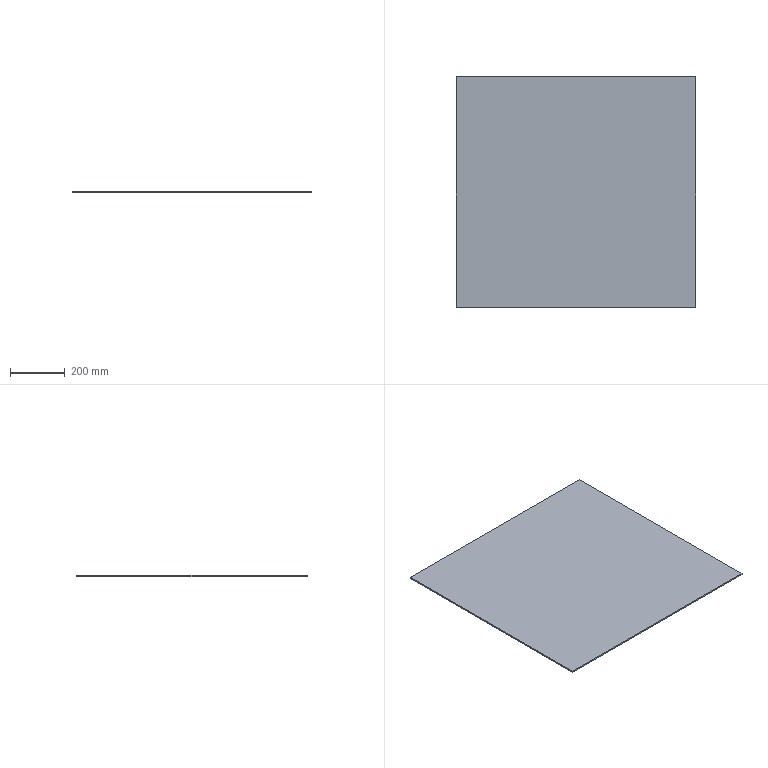Part | SolidWorks | features Extrusion 1, HoleWzd 1 | 1 solid | 6 faces | box 876 x 842 x 5 mm | volume 3687960 mm3 | plane 6
STEP:
#1=CARTESIAN_POINT('',(438.,-421.,0.));
#2=VERTEX_POINT('',#1);
#3=CARTESIAN_POINT('',(438.,421.,0.));
#4=VERTEX_POINT('',#3);
#5=CARTESIAN_POINT('',(438.,421.,0.));
#6=DIRECTION('',(0.,1.,0.));
#7=VECTOR('',#6,1000.);
#8=LINE('',#5,#7);
#9=EDGE_CURVE('',#2,#4,#8,.T.);
#10=ORIENTED_EDGE('',*,*,#9,.T.);
#11=CARTESIAN_POINT('',(438.,421.,5.));
#12=VERTEX_POINT('',#11);
#13=CARTESIAN_POINT('',(438.,421.,5.));
#14=DIRECTION('',(0.,0.,-1.));
#15=VECTOR('',#14,1000.);
#16=LINE('',#13,#15);
#17=EDGE_CURVE('',#12,#4,#16,.T.);
#18=ORIENTED_EDGE('',*,*,#17,.F.);
#19=CARTESIAN_POINT('',(438.,-421.,5.));
#20=VERTEX_POINT('',#19);
#21=CARTESIAN_POINT('',(438.,421.,5.));
#22=DIRECTION('',(0.,1.,0.));
#23=VECTOR('',#22,1000.);
#24=LINE('',#21,#23);
#25=EDGE_CURVE('',#20,#12,#24,.T.);
#26=ORIENTED_EDGE('',*,*,#25,.F.);
#27=CARTESIAN_POINT('',(438.,-421.,5.));
#28=DIRECTION('',(0.,0.,-1.));
#29=VECTOR('',#28,1000.);
#30=LINE('',#27,#29);
#31=EDGE_CURVE('',#20,#2,#30,.T.);
#32=ORIENTED_EDGE('',*,*,#31,.T.);
#33=EDGE_LOOP('',(#10,#18,#26,#32));
#34=FACE_OUTER_BOUND('',#33,.T.);
#35=CARTESIAN_POINT('',(438.,421.,5.));
#36=DIRECTION('',(-1.,0.,0.));
#37=DIRECTION('',(0.,-1.,0.));
#38=AXIS2_PLACEMENT_3D('',#35,#36,#37);
#39=PLANE('',#38);
#40=ADVANCED_FACE('',(#34),#39,.F.);
#41=CARTESIAN_POINT('',(-438.,421.,0.));
#42=VERTEX_POINT('',#41);
#43=CARTESIAN_POINT('',(-438.,421.,0.));
#44=DIRECTION('',(-1.,0.,0.));
#45=VECTOR('',#44,1000.);
#46=LINE('',#43,#45);
#47=EDGE_CURVE('',#4,#42,#46,.T.);
#48=ORIENTED_EDGE('',*,*,#47,.T.);
#49=CARTESIAN_POINT('',(-438.,421.,5.));
#50=VERTEX_POINT('',#49);
#51=CARTESIAN_POINT('',(-438.,421.,5.));
#52=DIRECTION('',(0.,0.,-1.));
#53=VECTOR('',#52,1000.);
#54=LINE('',#51,#53);
#55=EDGE_CURVE('',#50,#42,#54,.T.);
#56=ORIENTED_EDGE('',*,*,#55,.F.);
#57=CARTESIAN_POINT('',(-438.,421.,5.));
#58=DIRECTION('',(-1.,0.,0.));
#59=VECTOR('',#58,1000.);
#60=LINE('',#57,#59);
#61=EDGE_CURVE('',#12,#50,#60,.T.);
#62=ORIENTED_EDGE('',*,*,#61,.F.);
#63=ORIENTED_EDGE('',*,*,#17,.T.);
#64=EDGE_LOOP('',(#48,#56,#62,#63));
#65=FACE_OUTER_BOUND('',#64,.T.);
#66=CARTESIAN_POINT('',(-438.,421.,5.));
#67=DIRECTION('',(0.,-1.,0.));
#68=DIRECTION('',(0.,0.,-1.));
#69=AXIS2_PLACEMENT_3D('',#66,#67,#68);
#70=PLANE('',#69);
#71=ADVANCED_FACE('',(#65),#70,.F.);
#72=CARTESIAN_POINT('',(-438.,-421.,0.));
#73=VERTEX_POINT('',#72);
#74=CARTESIAN_POINT('',(-438.,421.,0.));
#75=DIRECTION('',(0.,-1.,0.));
#76=VECTOR('',#75,1000.);
#77=LINE('',#74,#76);
#78=EDGE_CURVE('',#42,#73,#77,.T.);
#79=ORIENTED_EDGE('',*,*,#78,.T.);
#80=CARTESIAN_POINT('',(-438.,-421.,5.));
#81=VERTEX_POINT('',#80);
#82=CARTESIAN_POINT('',(-438.,-421.,5.));
#83=DIRECTION('',(0.,0.,-1.));
#84=VECTOR('',#83,1000.);
#85=LINE('',#82,#84);
#86=EDGE_CURVE('',#81,#73,#85,.T.);
#87=ORIENTED_EDGE('',*,*,#86,.F.);
#88=CARTESIAN_POINT('',(-438.,421.,5.));
#89=DIRECTION('',(0.,-1.,0.));
#90=VECTOR('',#89,1000.);
#91=LINE('',#88,#90);
#92=EDGE_CURVE('',#50,#81,#91,.T.);
#93=ORIENTED_EDGE('',*,*,#92,.F.);
#94=ORIENTED_EDGE('',*,*,#55,.T.);
#95=EDGE_LOOP('',(#79,#87,#93,#94));
#96=FACE_OUTER_BOUND('',#95,.T.);
#97=CARTESIAN_POINT('',(-438.,421.,5.));
#98=DIRECTION('',(1.,0.,0.));
#99=DIRECTION('',(0.,1.,0.));
#100=AXIS2_PLACEMENT_3D('',#97,#98,#99);
#101=PLANE('',#100);
#102=ADVANCED_FACE('',(#96),#101,.F.);
#103=CARTESIAN_POINT('',(-438.,-421.,0.));
#104=DIRECTION('',(1.,0.,0.));
#105=VECTOR('',#104,1000.);
#106=LINE('',#103,#105);
#107=EDGE_CURVE('',#73,#2,#106,.T.);
#108=ORIENTED_EDGE('',*,*,#107,.T.);
#109=ORIENTED_EDGE('',*,*,#31,.F.);
#110=CARTESIAN_POINT('',(-438.,-421.,5.));
#111=DIRECTION('',(1.,0.,0.));
#112=VECTOR('',#111,1000.);
#113=LINE('',#110,#112);
#114=EDGE_CURVE('',#81,#20,#113,.T.);
#115=ORIENTED_EDGE('',*,*,#114,.F.);
#116=ORIENTED_EDGE('',*,*,#86,.T.);
#117=EDGE_LOOP('',(#108,#109,#115,#116));
#118=FACE_OUTER_BOUND('',#117,.T.);
#119=CARTESIAN_POINT('',(-438.,-421.,5.));
#120=DIRECTION('',(0.,1.,0.));
#121=DIRECTION('',(0.,0.,1.));
#122=AXIS2_PLACEMENT_3D('',#119,#120,#121);
#123=PLANE('',#122);
#124=ADVANCED_FACE('',(#118),#123,.F.);
#125=ORIENTED_EDGE('',*,*,#25,.T.);
#126=ORIENTED_EDGE('',*,*,#61,.T.);
#127=ORIENTED_EDGE('',*,*,#92,.T.);
#128=ORIENTED_EDGE('',*,*,#114,.T.);
#129=EDGE_LOOP('',(#125,#126,#127,#128));
#130=FACE_OUTER_BOUND('',#129,.T.);
#131=CARTESIAN_POINT('',(0.,0.,5.));
#132=DIRECTION('',(0.,0.,1.));
#133=DIRECTION('',(1.,0.,0.));
#134=AXIS2_PLACEMENT_3D('',#131,#132,#133);
#135=PLANE('',#134);
#136=ADVANCED_FACE('',(#130),#135,.T.);
#137=ORIENTED_EDGE('',*,*,#9,.F.);
#138=ORIENTED_EDGE('',*,*,#107,.F.);
#139=ORIENTED_EDGE('',*,*,#78,.F.);
#140=ORIENTED_EDGE('',*,*,#47,.F.);
#141=EDGE_LOOP('',(#137,#138,#139,#140));
#142=FACE_OUTER_BOUND('',#141,.T.);
#143=CARTESIAN_POINT('',(0.,0.,0.));
#144=DIRECTION('',(0.,0.,1.));
#145=DIRECTION('',(1.,0.,0.));
#146=AXIS2_PLACEMENT_3D('',#143,#144,#145);
#147=PLANE('',#146);
#148=ADVANCED_FACE('',(#142),#147,.F.);
#149=CLOSED_SHELL('',(#40,#71,#102,#124,#136,#148));
#150=MANIFOLD_SOLID_BREP('',#149);
#151=CARTESIAN_POINT('',(0.,0.,0.));
#152=DIRECTION('',(0.,0.,1.));
#153=DIRECTION('',(1.,0.,0.));
#154=AXIS2_PLACEMENT_3D('',#151,#152,#153);
#155=(LENGTH_UNIT()NAMED_UNIT(*)SI_UNIT(.MILLI.,.METRE.));
#156=UNCERTAINTY_MEASURE_WITH_UNIT(LENGTH_MEASURE(0.00001),#155,'','');
#157=(NAMED_UNIT(*)PLANE_ANGLE_UNIT()SI_UNIT($,.RADIAN.));
#158=(NAMED_UNIT(*)SI_UNIT($,.STERADIAN.)SOLID_ANGLE_UNIT());
#159=(GEOMETRIC_REPRESENTATION_CONTEXT(3)GLOBAL_UNCERTAINTY_ASSIGNED_CONTEXT((#156))GLOBAL_UNIT_ASSIGNED_CONTEXT((#155,#157,#158))REPRESENTATION_CONTEXT('',''));
#160=ADVANCED_BREP_SHAPE_REPRESENTATION('',(#150,#154),#159);